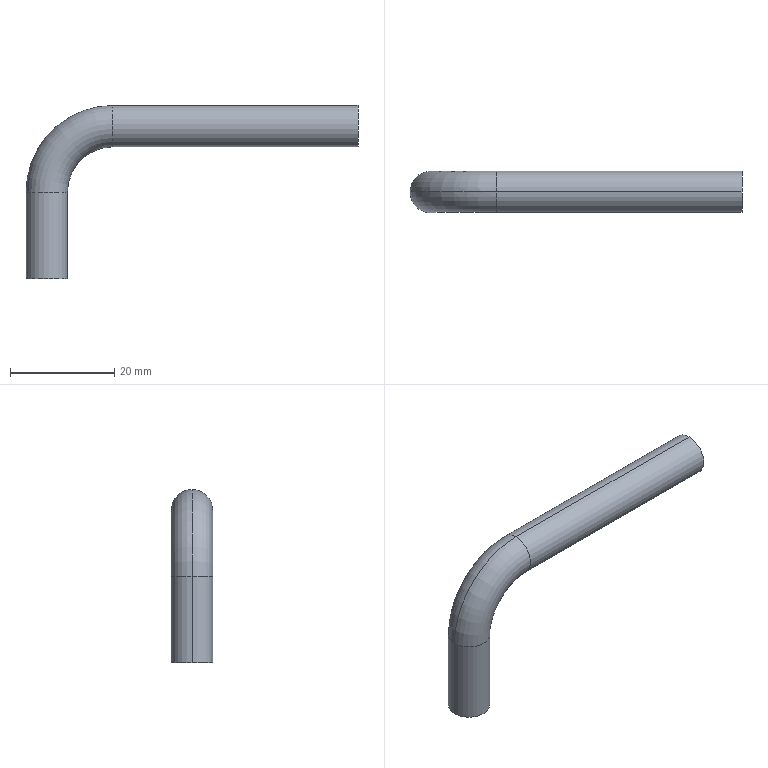Part | NX | features BREP 1 | 1 solid | 8 faces | box 63.659 x 7.938 x 33.179 mm | volume 4129 mm3 | cylinder 4 | plane 2 | torus 2 | commonest cylinder face diameters 7.938 x4
STEP:
#1=CARTESIAN_POINT('',(-3.969,0.,-29.21));
#2=VERTEX_POINT('',#1);
#3=CARTESIAN_POINT('',(3.969,0.,-29.21));
#4=VERTEX_POINT('',#3);
#5=CARTESIAN_POINT('',(0.,0.,-29.21));
#6=DIRECTION('',(0.,0.,1.));
#7=DIRECTION('',(-1.,0.,0.));
#8=AXIS2_PLACEMENT_3D('',#5,#6,#7);
#9=CIRCLE('',#8,3.969);
#10=EDGE_CURVE('',#2,#4,#9,.T.);
#11=ORIENTED_EDGE('',*,*,#10,.F.);
#12=CARTESIAN_POINT('',(0.,0.,-29.21));
#13=DIRECTION('',(0.,0.,1.));
#14=DIRECTION('',(1.,0.,0.));
#15=AXIS2_PLACEMENT_3D('',#12,#13,#14);
#16=CIRCLE('',#15,3.969);
#17=EDGE_CURVE('',#4,#2,#16,.T.);
#18=ORIENTED_EDGE('',*,*,#17,.F.);
#19=EDGE_LOOP('',(#11,#18));
#20=FACE_BOUND('',#19,.T.);
#21=CARTESIAN_POINT('',(0.,0.,-29.21));
#22=DIRECTION('',(0.,0.,1.));
#23=DIRECTION('',(1.,0.,0.));
#24=AXIS2_PLACEMENT_3D('',#21,#22,#23);
#25=PLANE('',#24);
#26=ADVANCED_FACE('',(#20),#25,.F.);
#27=CARTESIAN_POINT('',(-3.969,0.,-12.7));
#28=VERTEX_POINT('',#27);
#29=CARTESIAN_POINT('',(-3.969,0.,-29.21));
#30=DIRECTION('',(0.,0.,1.));
#31=VECTOR('',#30,1000.);
#32=LINE('',#29,#31);
#33=EDGE_CURVE('',#2,#28,#32,.T.);
#34=ORIENTED_EDGE('',*,*,#33,.T.);
#35=CARTESIAN_POINT('',(3.969,0.,-12.7));
#36=VERTEX_POINT('',#35);
#37=CARTESIAN_POINT('',(0.,0.,-12.7));
#38=DIRECTION('',(0.,0.,1.));
#39=DIRECTION('',(1.,0.,0.));
#40=AXIS2_PLACEMENT_3D('',#37,#38,#39);
#41=CIRCLE('',#40,3.969);
#42=EDGE_CURVE('',#36,#28,#41,.T.);
#43=ORIENTED_EDGE('',*,*,#42,.F.);
#44=CARTESIAN_POINT('',(3.969,0.,-29.21));
#45=DIRECTION('',(0.,0.,1.));
#46=VECTOR('',#45,1000.);
#47=LINE('',#44,#46);
#48=EDGE_CURVE('',#4,#36,#47,.T.);
#49=ORIENTED_EDGE('',*,*,#48,.F.);
#50=ORIENTED_EDGE('',*,*,#17,.T.);
#51=EDGE_LOOP('',(#34,#43,#49,#50));
#52=FACE_BOUND('',#51,.T.);
#53=CARTESIAN_POINT('',(0.,0.,-29.21));
#54=DIRECTION('',(0.,0.,1.));
#55=DIRECTION('',(1.,0.,0.));
#56=AXIS2_PLACEMENT_3D('',#53,#54,#55);
#57=CYLINDRICAL_SURFACE('',#56,3.969);
#58=ADVANCED_FACE('',(#52),#57,.T.);
#59=ORIENTED_EDGE('',*,*,#48,.T.);
#60=CARTESIAN_POINT('',(0.,0.,-12.7));
#61=DIRECTION('',(0.,0.,1.));
#62=DIRECTION('',(-1.,0.,0.));
#63=AXIS2_PLACEMENT_3D('',#60,#61,#62);
#64=CIRCLE('',#63,3.969);
#65=EDGE_CURVE('',#28,#36,#64,.T.);
#66=ORIENTED_EDGE('',*,*,#65,.F.);
#67=ORIENTED_EDGE('',*,*,#33,.F.);
#68=ORIENTED_EDGE('',*,*,#10,.T.);
#69=EDGE_LOOP('',(#59,#66,#67,#68));
#70=FACE_BOUND('',#69,.T.);
#71=CARTESIAN_POINT('',(0.,0.,-29.21));
#72=DIRECTION('',(0.,0.,1.));
#73=DIRECTION('',(1.,0.,0.));
#74=AXIS2_PLACEMENT_3D('',#71,#72,#73);
#75=CYLINDRICAL_SURFACE('',#74,3.969);
#76=ADVANCED_FACE('',(#70),#75,.T.);
#77=CARTESIAN_POINT('',(12.7,0.,-3.969));
#78=VERTEX_POINT('',#77);
#79=CARTESIAN_POINT('',(12.7,0.,-12.7));
#80=DIRECTION('',(0.,1.,0.));
#81=DIRECTION('',(-1.,0.,0.));
#82=AXIS2_PLACEMENT_3D('',#79,#80,#81);
#83=CIRCLE('',#82,8.731);
#84=EDGE_CURVE('',#78,#36,#83,.F.);
#85=ORIENTED_EDGE('',*,*,#84,.F.);
#86=CARTESIAN_POINT('',(12.7,0.,3.969));
#87=VERTEX_POINT('',#86);
#88=CARTESIAN_POINT('',(12.7,0.,0.));
#89=DIRECTION('',(1.,0.,0.));
#90=DIRECTION('',(0.,0.,1.));
#91=AXIS2_PLACEMENT_3D('',#88,#89,#90);
#92=CIRCLE('',#91,3.969);
#93=EDGE_CURVE('',#87,#78,#92,.T.);
#94=ORIENTED_EDGE('',*,*,#93,.F.);
#95=CARTESIAN_POINT('',(12.7,0.,-12.7));
#96=DIRECTION('',(0.,1.,0.));
#97=DIRECTION('',(-1.,0.,0.));
#98=AXIS2_PLACEMENT_3D('',#95,#96,#97);
#99=CIRCLE('',#98,16.669);
#100=EDGE_CURVE('',#87,#28,#99,.F.);
#101=ORIENTED_EDGE('',*,*,#100,.T.);
#102=ORIENTED_EDGE('',*,*,#65,.T.);
#103=EDGE_LOOP('',(#85,#94,#101,#102));
#104=FACE_BOUND('',#103,.T.);
#105=CARTESIAN_POINT('',(12.7,0.,-12.7));
#106=DIRECTION('',(0.,1.,0.));
#107=DIRECTION('',(1.,0.,0.));
#108=AXIS2_PLACEMENT_3D('',#105,#106,#107);
#109=TOROIDAL_SURFACE('',#108,12.7,3.969);
#110=ADVANCED_FACE('',(#104),#109,.T.);
#111=ORIENTED_EDGE('',*,*,#100,.F.);
#112=CARTESIAN_POINT('',(12.7,0.,0.));
#113=DIRECTION('',(1.,0.,0.));
#114=DIRECTION('',(0.,0.,-1.));
#115=AXIS2_PLACEMENT_3D('',#112,#113,#114);
#116=CIRCLE('',#115,3.969);
#117=EDGE_CURVE('',#78,#87,#116,.T.);
#118=ORIENTED_EDGE('',*,*,#117,.F.);
#119=ORIENTED_EDGE('',*,*,#84,.T.);
#120=ORIENTED_EDGE('',*,*,#42,.T.);
#121=EDGE_LOOP('',(#111,#118,#119,#120));
#122=FACE_BOUND('',#121,.T.);
#123=CARTESIAN_POINT('',(12.7,0.,-12.7));
#124=DIRECTION('',(0.,1.,0.));
#125=DIRECTION('',(1.,0.,0.));
#126=AXIS2_PLACEMENT_3D('',#123,#124,#125);
#127=TOROIDAL_SURFACE('',#126,12.7,3.969);
#128=ADVANCED_FACE('',(#122),#127,.T.);
#129=CARTESIAN_POINT('',(59.69,0.,3.969));
#130=VERTEX_POINT('',#129);
#131=CARTESIAN_POINT('',(12.7,0.,3.969));
#132=DIRECTION('',(1.,0.,0.));
#133=VECTOR('',#132,1000.);
#134=LINE('',#131,#133);
#135=EDGE_CURVE('',#130,#87,#134,.F.);
#136=ORIENTED_EDGE('',*,*,#135,.F.);
#137=CARTESIAN_POINT('',(59.69,0.,-3.969));
#138=VERTEX_POINT('',#137);
#139=CARTESIAN_POINT('',(59.69,0.,0.));
#140=DIRECTION('',(1.,0.,0.));
#141=DIRECTION('',(0.,0.,-1.));
#142=AXIS2_PLACEMENT_3D('',#139,#140,#141);
#143=CIRCLE('',#142,3.969);
#144=EDGE_CURVE('',#138,#130,#143,.T.);
#145=ORIENTED_EDGE('',*,*,#144,.F.);
#146=CARTESIAN_POINT('',(12.7,0.,-3.969));
#147=DIRECTION('',(1.,0.,0.));
#148=VECTOR('',#147,1000.);
#149=LINE('',#146,#148);
#150=EDGE_CURVE('',#138,#78,#149,.F.);
#151=ORIENTED_EDGE('',*,*,#150,.T.);
#152=ORIENTED_EDGE('',*,*,#117,.T.);
#153=EDGE_LOOP('',(#136,#145,#151,#152));
#154=FACE_BOUND('',#153,.T.);
#155=CARTESIAN_POINT('',(12.7,0.,0.));
#156=DIRECTION('',(1.,0.,0.));
#157=DIRECTION('',(0.,0.,-1.));
#158=AXIS2_PLACEMENT_3D('',#155,#156,#157);
#159=CYLINDRICAL_SURFACE('',#158,3.969);
#160=ADVANCED_FACE('',(#154),#159,.T.);
#161=ORIENTED_EDGE('',*,*,#150,.F.);
#162=CARTESIAN_POINT('',(59.69,0.,0.));
#163=DIRECTION('',(1.,0.,0.));
#164=DIRECTION('',(0.,0.,1.));
#165=AXIS2_PLACEMENT_3D('',#162,#163,#164);
#166=CIRCLE('',#165,3.969);
#167=EDGE_CURVE('',#130,#138,#166,.T.);
#168=ORIENTED_EDGE('',*,*,#167,.F.);
#169=ORIENTED_EDGE('',*,*,#135,.T.);
#170=ORIENTED_EDGE('',*,*,#93,.T.);
#171=EDGE_LOOP('',(#161,#168,#169,#170));
#172=FACE_BOUND('',#171,.T.);
#173=CARTESIAN_POINT('',(12.7,0.,0.));
#174=DIRECTION('',(1.,0.,0.));
#175=DIRECTION('',(0.,0.,-1.));
#176=AXIS2_PLACEMENT_3D('',#173,#174,#175);
#177=CYLINDRICAL_SURFACE('',#176,3.969);
#178=ADVANCED_FACE('',(#172),#177,.T.);
#179=ORIENTED_EDGE('',*,*,#167,.T.);
#180=ORIENTED_EDGE('',*,*,#144,.T.);
#181=EDGE_LOOP('',(#179,#180));
#182=FACE_BOUND('',#181,.T.);
#183=CARTESIAN_POINT('',(59.69,0.,0.));
#184=DIRECTION('',(1.,0.,0.));
#185=DIRECTION('',(0.,1.,0.));
#186=AXIS2_PLACEMENT_3D('',#183,#184,#185);
#187=PLANE('',#186);
#188=ADVANCED_FACE('',(#182),#187,.T.);
#189=CLOSED_SHELL('',(#26,#58,#76,#110,#128,#160,#178,#188));
#190=MANIFOLD_SOLID_BREP('',#189);
#191=(LENGTH_UNIT()NAMED_UNIT(*)SI_UNIT(.MILLI.,.METRE.));
#192=UNCERTAINTY_MEASURE_WITH_UNIT(LENGTH_MEASURE(0.00001),#191,'','');
#193=(NAMED_UNIT(*)PLANE_ANGLE_UNIT()SI_UNIT($,.RADIAN.));
#194=(NAMED_UNIT(*)SI_UNIT($,.STERADIAN.)SOLID_ANGLE_UNIT());
#195=(GEOMETRIC_REPRESENTATION_CONTEXT(3)GLOBAL_UNCERTAINTY_ASSIGNED_CONTEXT((#192))GLOBAL_UNIT_ASSIGNED_CONTEXT((#191,#193,#194))REPRESENTATION_CONTEXT('',''));
#196=ADVANCED_BREP_SHAPE_REPRESENTATION('',(#190),#195);